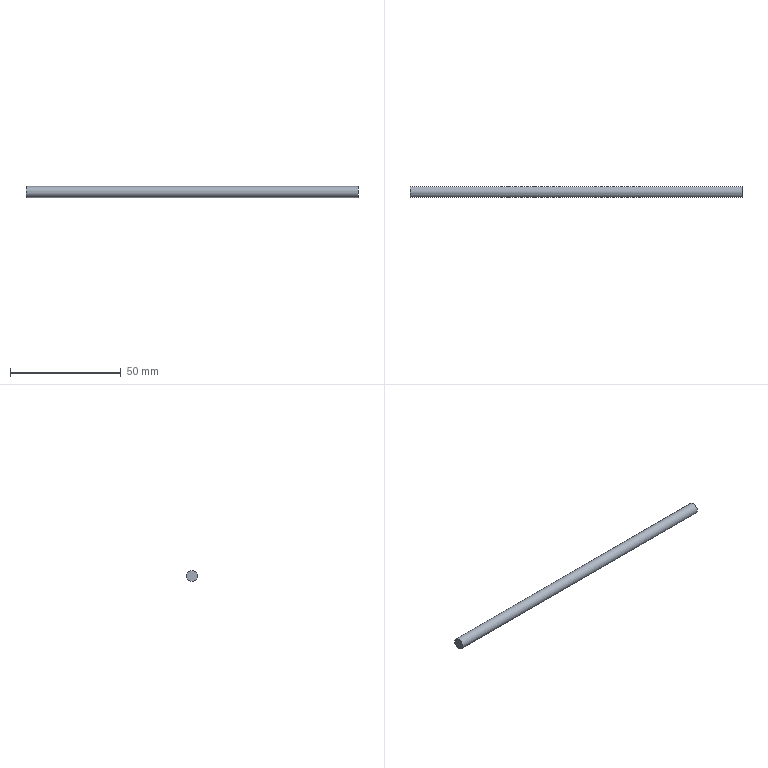Part | NX | features solid 2 | 1 solid | 3 faces | box 150 x 5 x 5 mm | volume 2945 mm3 | plane 2 | cylinder 1 | commonest cylinder face diameters 5 x1
STEP:
#1=CARTESIAN_POINT('',(637.,377.5,-372.5));
#2=VERTEX_POINT('',#1);
#3=CARTESIAN_POINT('',(637.,377.5,-375.));
#4=DIRECTION('',(-1.,0.,0.));
#5=DIRECTION('',(0.,0.,1.));
#6=AXIS2_PLACEMENT_3D('',#3,#4,#5);
#7=CIRCLE('',#6,2.5);
#8=EDGE_CURVE('',#2,#2,#7,.T.);
#9=ORIENTED_EDGE('',*,*,#8,.F.);
#10=EDGE_LOOP('',(#9));
#11=FACE_BOUND('',#10,.T.);
#12=CARTESIAN_POINT('',(787.,377.5,-372.5));
#13=VERTEX_POINT('',#12);
#14=CARTESIAN_POINT('',(787.,377.5,-375.));
#15=DIRECTION('',(-1.,0.,0.));
#16=DIRECTION('',(0.,0.,1.));
#17=AXIS2_PLACEMENT_3D('',#14,#15,#16);
#18=CIRCLE('',#17,2.5);
#19=EDGE_CURVE('',#13,#13,#18,.T.);
#20=ORIENTED_EDGE('',*,*,#19,.T.);
#21=EDGE_LOOP('',(#20));
#22=FACE_BOUND('',#21,.T.);
#23=CARTESIAN_POINT('',(637.,377.5,-375.));
#24=DIRECTION('',(1.,0.,0.));
#25=DIRECTION('',(0.,0.,-1.));
#26=AXIS2_PLACEMENT_3D('',#23,#24,#25);
#27=CYLINDRICAL_SURFACE('',#26,2.5);
#28=ADVANCED_FACE('',(#11,#22),#27,.T.);
#29=ORIENTED_EDGE('',*,*,#8,.T.);
#30=EDGE_LOOP('',(#29));
#31=FACE_BOUND('',#30,.T.);
#32=CARTESIAN_POINT('',(637.,377.5,-375.));
#33=DIRECTION('',(-1.,0.,0.));
#34=DIRECTION('',(0.,0.,1.));
#35=AXIS2_PLACEMENT_3D('',#32,#33,#34);
#36=PLANE('',#35);
#37=ADVANCED_FACE('',(#31),#36,.T.);
#38=ORIENTED_EDGE('',*,*,#19,.F.);
#39=EDGE_LOOP('',(#38));
#40=FACE_BOUND('',#39,.T.);
#41=CARTESIAN_POINT('',(787.,377.5,-375.));
#42=DIRECTION('',(-1.,0.,0.));
#43=DIRECTION('',(0.,0.,1.));
#44=AXIS2_PLACEMENT_3D('',#41,#42,#43);
#45=PLANE('',#44);
#46=ADVANCED_FACE('',(#40),#45,.F.);
#47=CLOSED_SHELL('',(#28,#37,#46));
#48=MANIFOLD_SOLID_BREP('',#47);
#49=(LENGTH_UNIT()NAMED_UNIT(*)SI_UNIT(.MILLI.,.METRE.));
#50=UNCERTAINTY_MEASURE_WITH_UNIT(LENGTH_MEASURE(0.00001),#49,'','');
#51=(NAMED_UNIT(*)PLANE_ANGLE_UNIT()SI_UNIT($,.RADIAN.));
#52=(NAMED_UNIT(*)SI_UNIT($,.STERADIAN.)SOLID_ANGLE_UNIT());
#53=(GEOMETRIC_REPRESENTATION_CONTEXT(3)GLOBAL_UNCERTAINTY_ASSIGNED_CONTEXT((#50))GLOBAL_UNIT_ASSIGNED_CONTEXT((#49,#51,#52))REPRESENTATION_CONTEXT('',''));
#54=ADVANCED_BREP_SHAPE_REPRESENTATION('',(#48),#53);